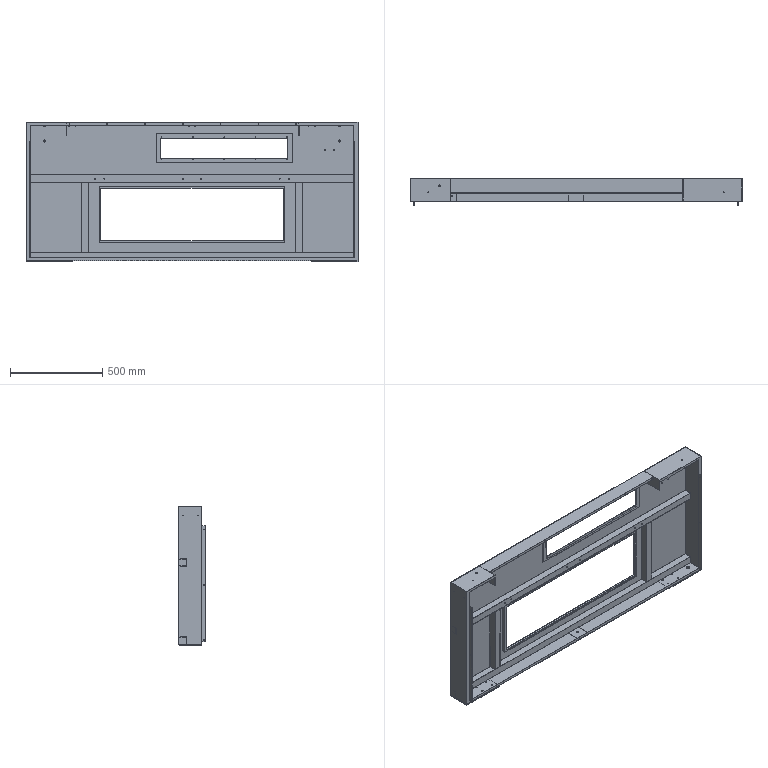Part | STEP file | 9 solids | 285 faces | box 1800 x 145 x 755 mm | volume 4684441 mm3 | cylinder 152 | plane 129 | cone 4 | commonest cylinder face diameters 6.8 x44 4.2 x24 3.3 x20 12 x16 3.2 x14 5.2 x12